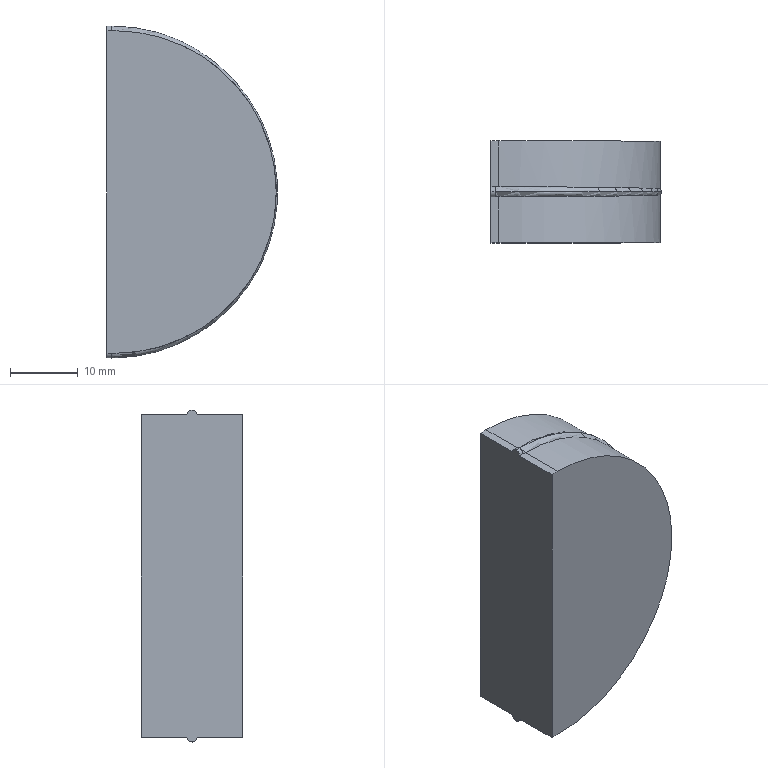Part | STEP file | OP10-148_seal block | 1 solid | 18 faces | box 25.2 x 15 x 49 mm | volume 13850 mm3 | cylinder 8 | torus 6 | plane 4 | commonest cylinder face diameters 47.6 x6 9 x2